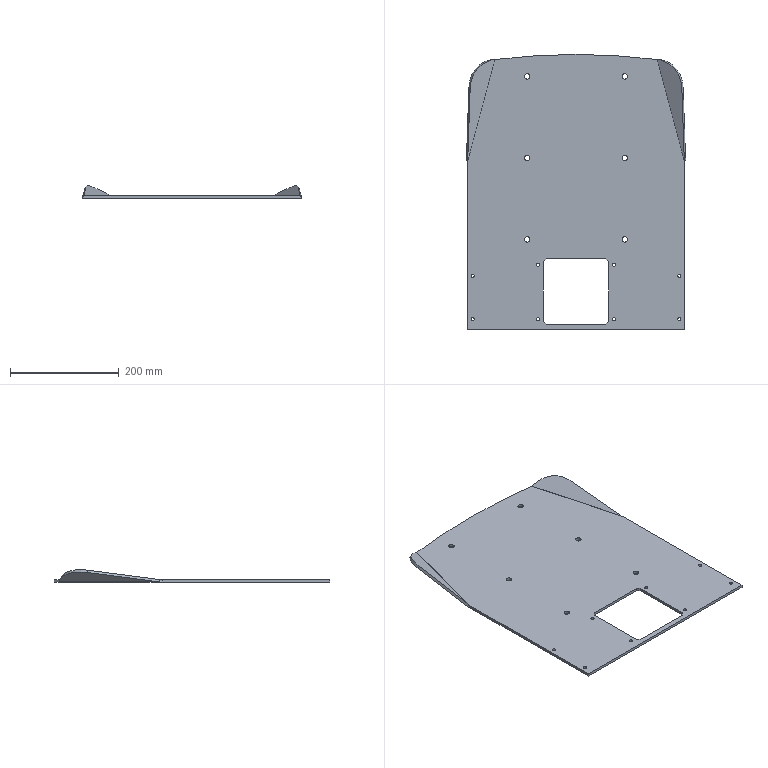Part | SolidWorks | features ICE 5, HoleWzd 2, Chamfer 1, EdgeFlange 1, Fillet 1, FlatPattern 1, SM3dBend 1, SMBaseFlange 1, SheetMetal 1 | 1 solid | 60 faces | box 403.29 x 506.284 x 23.281 mm | volume 923449 mm3 | cylinder 37 | plane 19 | spline 4 | commonest cylinder face diameters 5.8 x16 10 x12 2400 x3 1 x2 11 x2 100 x2